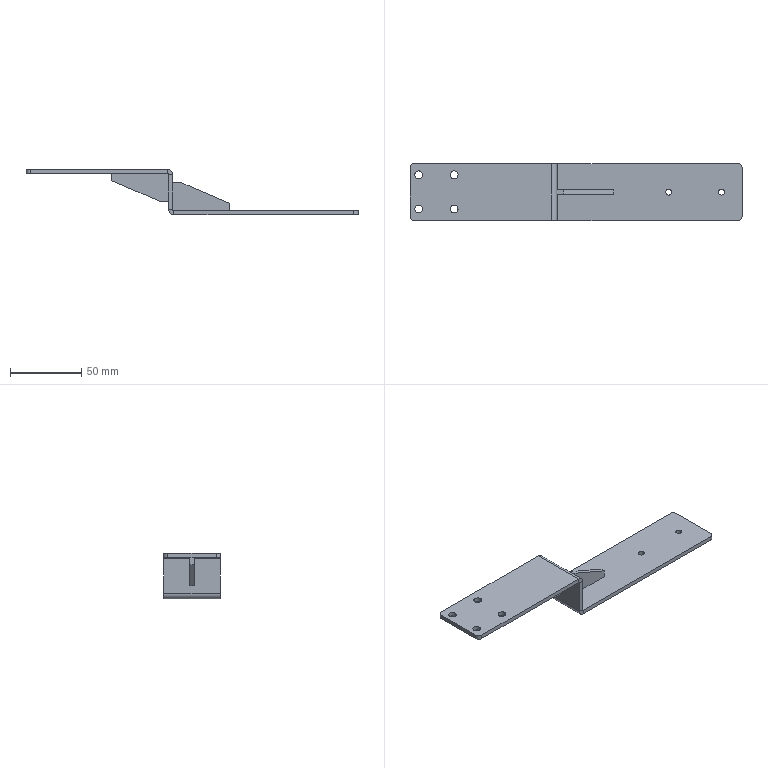Part | SolidWorks | features HoleWzd 2, ICE 2, Fillet 1, FlatPattern 1, SMBaseFlange 1, SheetMetal 1 | 1 solid | 50 faces | box 233 x 40 x 32 mm | volume 34041 mm3 | plane 28 | cylinder 22 | commonest cylinder face diameters 5.5 x8 1.5 x4 4.2 x4 6 x4 7.5 x2
STEP:
#1=CARTESIAN_POINT('',(8.75,8.,0.));
#2=VERTEX_POINT('',#1);
#3=CARTESIAN_POINT('',(3.25,8.,0.));
#4=VERTEX_POINT('',#3);
#5=CARTESIAN_POINT('',(6.,8.,0.));
#6=DIRECTION('',(0.,0.,-1.));
#7=DIRECTION('',(-1.,0.,0.));
#8=AXIS2_PLACEMENT_3D('',#5,#6,#7);
#9=CIRCLE('',#8,2.75);
#10=EDGE_CURVE('',#2,#4,#9,.T.);
#11=ORIENTED_EDGE('',*,*,#10,.T.);
#12=CARTESIAN_POINT('',(3.25,8.,3.));
#13=VERTEX_POINT('',#12);
#14=CARTESIAN_POINT('',(3.25,8.,3.));
#15=DIRECTION('',(0.,0.,1.));
#16=VECTOR('',#15,1000.);
#17=LINE('',#14,#16);
#18=EDGE_CURVE('',#4,#13,#17,.T.);
#19=ORIENTED_EDGE('',*,*,#18,.T.);
#20=CARTESIAN_POINT('',(8.75,8.,3.));
#21=VERTEX_POINT('',#20);
#22=CARTESIAN_POINT('',(6.,8.,3.));
#23=DIRECTION('',(0.,0.,1.));
#24=DIRECTION('',(1.,0.,0.));
#25=AXIS2_PLACEMENT_3D('',#22,#23,#24);
#26=CIRCLE('',#25,2.75);
#27=EDGE_CURVE('',#13,#21,#26,.T.);
#28=ORIENTED_EDGE('',*,*,#27,.T.);
#29=CARTESIAN_POINT('',(8.75,8.,3.));
#30=DIRECTION('',(0.,0.,1.));
#31=VECTOR('',#30,1000.);
#32=LINE('',#29,#31);
#33=EDGE_CURVE('',#2,#21,#32,.T.);
#34=ORIENTED_EDGE('',*,*,#33,.F.);
#35=EDGE_LOOP('',(#11,#19,#28,#34));
#36=FACE_OUTER_BOUND('',#35,.T.);
#37=CARTESIAN_POINT('',(6.,8.,3.));
#38=DIRECTION('',(0.,0.,1.));
#39=DIRECTION('',(1.,0.,0.));
#40=AXIS2_PLACEMENT_3D('',#37,#38,#39);
#41=CYLINDRICAL_SURFACE('',#40,2.75);
#42=ADVANCED_FACE('',(#36),#41,.F.);
#43=CARTESIAN_POINT('',(8.75,32.,0.));
#44=VERTEX_POINT('',#43);
#45=CARTESIAN_POINT('',(3.25,32.,0.));
#46=VERTEX_POINT('',#45);
#47=CARTESIAN_POINT('',(6.,32.,0.));
#48=DIRECTION('',(0.,0.,-1.));
#49=DIRECTION('',(-1.,0.,0.));
#50=AXIS2_PLACEMENT_3D('',#47,#48,#49);
#51=CIRCLE('',#50,2.75);
#52=EDGE_CURVE('',#44,#46,#51,.T.);
#53=ORIENTED_EDGE('',*,*,#52,.T.);
#54=CARTESIAN_POINT('',(3.25,32.,3.));
#55=VERTEX_POINT('',#54);
#56=CARTESIAN_POINT('',(3.25,32.,3.));
#57=DIRECTION('',(0.,0.,1.));
#58=VECTOR('',#57,1000.);
#59=LINE('',#56,#58);
#60=EDGE_CURVE('',#46,#55,#59,.T.);
#61=ORIENTED_EDGE('',*,*,#60,.T.);
#62=CARTESIAN_POINT('',(8.75,32.,3.));
#63=VERTEX_POINT('',#62);
#64=CARTESIAN_POINT('',(6.,32.,3.));
#65=DIRECTION('',(0.,0.,1.));
#66=DIRECTION('',(1.,0.,0.));
#67=AXIS2_PLACEMENT_3D('',#64,#65,#66);
#68=CIRCLE('',#67,2.75);
#69=EDGE_CURVE('',#55,#63,#68,.T.);
#70=ORIENTED_EDGE('',*,*,#69,.T.);
#71=CARTESIAN_POINT('',(8.75,32.,3.));
#72=DIRECTION('',(0.,0.,1.));
#73=VECTOR('',#72,1000.);
#74=LINE('',#71,#73);
#75=EDGE_CURVE('',#44,#63,#74,.T.);
#76=ORIENTED_EDGE('',*,*,#75,.F.);
#77=EDGE_LOOP('',(#53,#61,#70,#76));
#78=FACE_OUTER_BOUND('',#77,.T.);
#79=CARTESIAN_POINT('',(6.,32.,3.));
#80=DIRECTION('',(0.,0.,1.));
#81=DIRECTION('',(1.,0.,0.));
#82=AXIS2_PLACEMENT_3D('',#79,#80,#81);
#83=CYLINDRICAL_SURFACE('',#82,2.75);
#84=ADVANCED_FACE('',(#78),#83,.F.);
#85=CARTESIAN_POINT('',(33.75,8.,0.));
#86=VERTEX_POINT('',#85);
#87=CARTESIAN_POINT('',(28.25,8.,0.));
#88=VERTEX_POINT('',#87);
#89=CARTESIAN_POINT('',(31.,8.,0.));
#90=DIRECTION('',(0.,0.,-1.));
#91=DIRECTION('',(-1.,0.,0.));
#92=AXIS2_PLACEMENT_3D('',#89,#90,#91);
#93=CIRCLE('',#92,2.75);
#94=EDGE_CURVE('',#86,#88,#93,.T.);
#95=ORIENTED_EDGE('',*,*,#94,.T.);
#96=CARTESIAN_POINT('',(28.25,8.,3.));
#97=VERTEX_POINT('',#96);
#98=CARTESIAN_POINT('',(28.25,8.,3.));
#99=DIRECTION('',(0.,0.,1.));
#100=VECTOR('',#99,1000.);
#101=LINE('',#98,#100);
#102=EDGE_CURVE('',#88,#97,#101,.T.);
#103=ORIENTED_EDGE('',*,*,#102,.T.);
#104=CARTESIAN_POINT('',(33.75,8.,3.));
#105=VERTEX_POINT('',#104);
#106=CARTESIAN_POINT('',(31.,8.,3.));
#107=DIRECTION('',(0.,0.,1.));
#108=DIRECTION('',(1.,0.,0.));
#109=AXIS2_PLACEMENT_3D('',#106,#107,#108);
#110=CIRCLE('',#109,2.75);
#111=EDGE_CURVE('',#97,#105,#110,.T.);
#112=ORIENTED_EDGE('',*,*,#111,.T.);
#113=CARTESIAN_POINT('',(33.75,8.,3.));
#114=DIRECTION('',(0.,0.,1.));
#115=VECTOR('',#114,1000.);
#116=LINE('',#113,#115);
#117=EDGE_CURVE('',#86,#105,#116,.T.);
#118=ORIENTED_EDGE('',*,*,#117,.F.);
#119=EDGE_LOOP('',(#95,#103,#112,#118));
#120=FACE_OUTER_BOUND('',#119,.T.);
#121=CARTESIAN_POINT('',(31.,8.,3.));
#122=DIRECTION('',(0.,0.,1.));
#123=DIRECTION('',(1.,0.,0.));
#124=AXIS2_PLACEMENT_3D('',#121,#122,#123);
#125=CYLINDRICAL_SURFACE('',#124,2.75);
#126=ADVANCED_FACE('',(#120),#125,.F.);
#127=CARTESIAN_POINT('',(33.75,32.,0.));
#128=VERTEX_POINT('',#127);
#129=CARTESIAN_POINT('',(28.25,32.,0.));
#130=VERTEX_POINT('',#129);
#131=CARTESIAN_POINT('',(31.,32.,0.));
#132=DIRECTION('',(0.,0.,-1.));
#133=DIRECTION('',(-1.,0.,0.));
#134=AXIS2_PLACEMENT_3D('',#131,#132,#133);
#135=CIRCLE('',#134,2.75);
#136=EDGE_CURVE('',#128,#130,#135,.T.);
#137=ORIENTED_EDGE('',*,*,#136,.T.);
#138=CARTESIAN_POINT('',(28.25,32.,3.));
#139=VERTEX_POINT('',#138);
#140=CARTESIAN_POINT('',(28.25,32.,3.));
#141=DIRECTION('',(0.,0.,1.));
#142=VECTOR('',#141,1000.);
#143=LINE('',#140,#142);
#144=EDGE_CURVE('',#130,#139,#143,.T.);
#145=ORIENTED_EDGE('',*,*,#144,.T.);
#146=CARTESIAN_POINT('',(33.75,32.,3.));
#147=VERTEX_POINT('',#146);
#148=CARTESIAN_POINT('',(31.,32.,3.));
#149=DIRECTION('',(0.,0.,1.));
#150=DIRECTION('',(1.,0.,0.));
#151=AXIS2_PLACEMENT_3D('',#148,#149,#150);
#152=CIRCLE('',#151,2.75);
#153=EDGE_CURVE('',#139,#147,#152,.T.);
#154=ORIENTED_EDGE('',*,*,#153,.T.);
#155=CARTESIAN_POINT('',(33.75,32.,3.));
#156=DIRECTION('',(0.,0.,1.));
#157=VECTOR('',#156,1000.);
#158=LINE('',#155,#157);
#159=EDGE_CURVE('',#128,#147,#158,.T.);
#160=ORIENTED_EDGE('',*,*,#159,.F.);
#161=EDGE_LOOP('',(#137,#145,#154,#160));
#162=FACE_OUTER_BOUND('',#161,.T.);
#163=CARTESIAN_POINT('',(31.,32.,3.));
#164=DIRECTION('',(0.,0.,1.));
#165=DIRECTION('',(1.,0.,0.));
#166=AXIS2_PLACEMENT_3D('',#163,#164,#165);
#167=CYLINDRICAL_SURFACE('',#166,2.75);
#168=ADVANCED_FACE('',(#162),#167,.F.);
#169=CARTESIAN_POINT('',(220.65,20.,-29.));
#170=VERTEX_POINT('',#169);
#171=CARTESIAN_POINT('',(216.45,20.,-29.));
#172=VERTEX_POINT('',#171);
#173=CARTESIAN_POINT('',(218.55,20.,-29.));
#174=DIRECTION('',(0.,0.,-1.));
#175=DIRECTION('',(-1.,0.,0.));
#176=AXIS2_PLACEMENT_3D('',#173,#174,#175);
#177=CIRCLE('',#176,2.1);
#178=EDGE_CURVE('',#170,#172,#177,.T.);
#179=ORIENTED_EDGE('',*,*,#178,.T.);
#180=CARTESIAN_POINT('',(216.45,20.,-26.));
#181=VERTEX_POINT('',#180);
#182=CARTESIAN_POINT('',(216.45,20.,-26.));
#183=DIRECTION('',(0.,0.,1.));
#184=VECTOR('',#183,1000.);
#185=LINE('',#182,#184);
#186=EDGE_CURVE('',#172,#181,#185,.T.);
#187=ORIENTED_EDGE('',*,*,#186,.T.);
#188=CARTESIAN_POINT('',(220.65,20.,-26.));
#189=VERTEX_POINT('',#188);
#190=CARTESIAN_POINT('',(218.55,20.,-26.));
#191=DIRECTION('',(0.,0.,1.));
#192=DIRECTION('',(1.,0.,0.));
#193=AXIS2_PLACEMENT_3D('',#190,#191,#192);
#194=CIRCLE('',#193,2.1);
#195=EDGE_CURVE('',#181,#189,#194,.T.);
#196=ORIENTED_EDGE('',*,*,#195,.T.);
#197=CARTESIAN_POINT('',(220.65,20.,-26.));
#198=DIRECTION('',(0.,0.,1.));
#199=VECTOR('',#198,1000.);
#200=LINE('',#197,#199);
#201=EDGE_CURVE('',#170,#189,#200,.T.);
#202=ORIENTED_EDGE('',*,*,#201,.F.);
#203=EDGE_LOOP('',(#179,#187,#196,#202));
#204=FACE_OUTER_BOUND('',#203,.T.);
#205=CARTESIAN_POINT('',(218.55,20.,-26.));
#206=DIRECTION('',(0.,0.,1.));
#207=DIRECTION('',(1.,0.,0.));
#208=AXIS2_PLACEMENT_3D('',#205,#206,#207);
#209=CYLINDRICAL_SURFACE('',#208,2.1);
#210=ADVANCED_FACE('',(#204),#209,.F.);
#211=CARTESIAN_POINT('',(183.65,20.,-29.));
#212=VERTEX_POINT('',#211);
#213=CARTESIAN_POINT('',(179.45,20.,-29.));
#214=VERTEX_POINT('',#213);
#215=CARTESIAN_POINT('',(181.55,20.,-29.));
#216=DIRECTION('',(0.,0.,-1.));
#217=DIRECTION('',(-1.,0.,0.));
#218=AXIS2_PLACEMENT_3D('',#215,#216,#217);
#219=CIRCLE('',#218,2.1);
#220=EDGE_CURVE('',#212,#214,#219,.T.);
#221=ORIENTED_EDGE('',*,*,#220,.T.);
#222=CARTESIAN_POINT('',(179.45,20.,-26.));
#223=VERTEX_POINT('',#222);
#224=CARTESIAN_POINT('',(179.45,20.,-26.));
#225=DIRECTION('',(0.,0.,1.));
#226=VECTOR('',#225,1000.);
#227=LINE('',#224,#226);
#228=EDGE_CURVE('',#214,#223,#227,.T.);
#229=ORIENTED_EDGE('',*,*,#228,.T.);
#230=CARTESIAN_POINT('',(183.65,20.,-26.));
#231=VERTEX_POINT('',#230);
#232=CARTESIAN_POINT('',(181.55,20.,-26.));
#233=DIRECTION('',(0.,0.,1.));
#234=DIRECTION('',(1.,0.,0.));
#235=AXIS2_PLACEMENT_3D('',#232,#233,#234);
#236=CIRCLE('',#235,2.1);
#237=EDGE_CURVE('',#223,#231,#236,.T.);
#238=ORIENTED_EDGE('',*,*,#237,.T.);
#239=CARTESIAN_POINT('',(183.65,20.,-26.));
#240=DIRECTION('',(0.,0.,1.));
#241=VECTOR('',#240,1000.);
#242=LINE('',#239,#241);
#243=EDGE_CURVE('',#212,#231,#242,.T.);
#244=ORIENTED_EDGE('',*,*,#243,.F.);
#245=EDGE_LOOP('',(#221,#229,#238,#244));
#246=FACE_OUTER_BOUND('',#245,.T.);
#247=CARTESIAN_POINT('',(181.55,20.,-26.));
#248=DIRECTION('',(0.,0.,1.));
#249=DIRECTION('',(1.,0.,0.));
#250=AXIS2_PLACEMENT_3D('',#247,#248,#249);
#251=CYLINDRICAL_SURFACE('',#250,2.1);
#252=ADVANCED_FACE('',(#246),#251,.F.);
#253=CARTESIAN_POINT('',(103.75,18.5,-26.));
#254=VERTEX_POINT('',#253);
#255=CARTESIAN_POINT('',(103.,18.5,-25.25));
#256=VERTEX_POINT('',#255);
#257=CARTESIAN_POINT('',(103.75,18.5,-25.25));
#258=DIRECTION('',(0.,1.,0.));
#259=DIRECTION('',(0.,0.,1.));
#260=AXIS2_PLACEMENT_3D('',#257,#258,#259);
#261=CIRCLE('',#260,0.75);
#262=EDGE_CURVE('',#254,#256,#261,.T.);
#263=ORIENTED_EDGE('',*,*,#262,.T.);
#264=CARTESIAN_POINT('',(103.,0.,-25.25));
#265=VERTEX_POINT('',#264);
#266=CARTESIAN_POINT('',(103.,40.,-25.25));
#267=DIRECTION('',(0.,-1.,0.));
#268=VECTOR('',#267,1000.);
#269=LINE('',#266,#268);
#270=EDGE_CURVE('',#256,#265,#269,.T.);
#271=ORIENTED_EDGE('',*,*,#270,.T.);
#272=CARTESIAN_POINT('',(103.75,0.,-26.));
#273=VERTEX_POINT('',#272);
#274=CARTESIAN_POINT('',(103.75,0.,-25.25));
#275=DIRECTION('',(0.,-1.,0.));
#276=DIRECTION('',(1.,0.,0.));
#277=AXIS2_PLACEMENT_3D('',#274,#275,#276);
#278=CIRCLE('',#277,0.75);
#279=EDGE_CURVE('',#265,#273,#278,.T.);
#280=ORIENTED_EDGE('',*,*,#279,.T.);
#281=CARTESIAN_POINT('',(103.75,40.,-26.));
#282=DIRECTION('',(0.,-1.,0.));
#283=VECTOR('',#282,1000.);
#284=LINE('',#281,#283);
#285=EDGE_CURVE('',#254,#273,#284,.T.);
#286=ORIENTED_EDGE('',*,*,#285,.F.);
#287=EDGE_LOOP('',(#263,#271,#280,#286));
#288=FACE_OUTER_BOUND('',#287,.T.);
#289=CARTESIAN_POINT('',(103.75,40.,-25.25));
#290=DIRECTION('',(0.,-1.,0.));
#291=DIRECTION('',(0.,0.,-1.));
#292=AXIS2_PLACEMENT_3D('',#289,#290,#291);
#293=CYLINDRICAL_SURFACE('',#292,0.75);
#294=ADVANCED_FACE('',(#288),#293,.F.);
#295=CARTESIAN_POINT('',(99.25,18.5,0.));
#296=VERTEX_POINT('',#295);
#297=CARTESIAN_POINT('',(99.25,0.,0.));
#298=VERTEX_POINT('',#297);
#299=CARTESIAN_POINT('',(99.25,40.,0.));
#300=DIRECTION('',(0.,-1.,0.));
#301=VECTOR('',#300,1000.);
#302=LINE('',#299,#301);
#303=EDGE_CURVE('',#296,#298,#302,.T.);
#304=ORIENTED_EDGE('',*,*,#303,.F.);
#305=CARTESIAN_POINT('',(100.,18.5,-0.75));
#306=VERTEX_POINT('',#305);
#307=CARTESIAN_POINT('',(99.25,18.5,-0.75));
#308=DIRECTION('',(0.,1.,0.));
#309=DIRECTION('',(0.,0.,1.));
#310=AXIS2_PLACEMENT_3D('',#307,#308,#309);
#311=CIRCLE('',#310,0.75);
#312=EDGE_CURVE('',#296,#306,#311,.T.);
#313=ORIENTED_EDGE('',*,*,#312,.T.);
#314=CARTESIAN_POINT('',(100.,0.,-0.75));
#315=VERTEX_POINT('',#314);
#316=CARTESIAN_POINT('',(100.,40.,-0.75));
#317=DIRECTION('',(0.,-1.,0.));
#318=VECTOR('',#317,1000.);
#319=LINE('',#316,#318);
#320=EDGE_CURVE('',#306,#315,#319,.T.);
#321=ORIENTED_EDGE('',*,*,#320,.T.);
#322=CARTESIAN_POINT('',(99.25,0.,-0.75));
#323=DIRECTION('',(0.,1.,0.));
#324=DIRECTION('',(0.,0.,-1.));
#325=AXIS2_PLACEMENT_3D('',#322,#323,#324);
#326=CIRCLE('',#325,0.75);
#327=EDGE_CURVE('',#298,#315,#326,.T.);
#328=ORIENTED_EDGE('',*,*,#327,.F.);
#329=EDGE_LOOP('',(#304,#313,#321,#328));
#330=FACE_OUTER_BOUND('',#329,.T.);
#331=CARTESIAN_POINT('',(99.25,40.,-0.75));
#332=DIRECTION('',(0.,-1.,0.));
#333=DIRECTION('',(0.,0.,-1.));
#334=AXIS2_PLACEMENT_3D('',#331,#332,#333);
#335=CYLINDRICAL_SURFACE('',#334,0.75);
#336=ADVANCED_FACE('',(#330),#335,.F.);
#337=CARTESIAN_POINT('',(100.,40.,-0.75));
#338=VERTEX_POINT('',#337);
#339=CARTESIAN_POINT('',(103.,40.,-0.75));
#340=VERTEX_POINT('',#339);
#341=CARTESIAN_POINT('',(100.,40.,-0.75));
#342=DIRECTION('',(1.,0.,0.));
#343=VECTOR('',#342,1000.);
#344=LINE('',#341,#343);
#345=EDGE_CURVE('',#338,#340,#344,.T.);
#346=ORIENTED_EDGE('',*,*,#345,.F.);
#347=CARTESIAN_POINT('',(99.25,40.,0.));
#348=VERTEX_POINT('',#347);
#349=CARTESIAN_POINT('',(99.25,40.,-0.75));
#350=DIRECTION('',(0.,1.,0.));
#351=DIRECTION('',(0.,0.,-1.));
#352=AXIS2_PLACEMENT_3D('',#349,#350,#351);
#353=CIRCLE('',#352,0.75);
#354=EDGE_CURVE('',#348,#338,#353,.T.);
#355=ORIENTED_EDGE('',*,*,#354,.F.);
#356=CARTESIAN_POINT('',(99.25,40.,3.));
#357=VERTEX_POINT('',#356);
#358=CARTESIAN_POINT('',(99.25,40.,3.));
#359=DIRECTION('',(0.,0.,-1.));
#360=VECTOR('',#359,1000.);
#361=LINE('',#358,#360);
#362=EDGE_CURVE('',#357,#348,#361,.T.);
#363=ORIENTED_EDGE('',*,*,#362,.F.);
#364=CARTESIAN_POINT('',(99.25,40.,-0.75));
#365=DIRECTION('',(0.,1.,0.));
#366=DIRECTION('',(1.,0.,0.));
#367=AXIS2_PLACEMENT_3D('',#364,#365,#366);
#368=CIRCLE('',#367,3.75);
#369=EDGE_CURVE('',#357,#340,#368,.T.);
#370=ORIENTED_EDGE('',*,*,#369,.T.);
#371=EDGE_LOOP('',(#346,#355,#363,#370));
#372=FACE_OUTER_BOUND('',#371,.T.);
#373=CARTESIAN_POINT('',(100.,40.,-0.75));
#374=DIRECTION('',(0.,1.,0.));
#375=DIRECTION('',(0.,0.,1.));
#376=AXIS2_PLACEMENT_3D('',#373,#374,#375);
#377=PLANE('',#376);
#378=ADVANCED_FACE('',(#372),#377,.T.);
#379=CARTESIAN_POINT('',(100.,40.,-25.25));
#380=VERTEX_POINT('',#379);
#381=CARTESIAN_POINT('',(100.,40.,0.));
#382=DIRECTION('',(0.,0.,-1.));
#383=VECTOR('',#382,1000.);
#384=LINE('',#381,#383);
#385=EDGE_CURVE('',#338,#380,#384,.T.);
#386=ORIENTED_EDGE('',*,*,#385,.F.);
#387=ORIENTED_EDGE('',*,*,#345,.T.);
#388=CARTESIAN_POINT('',(103.,40.,-25.25));
#389=VERTEX_POINT('',#388);
#390=CARTESIAN_POINT('',(103.,40.,0.));
#391=DIRECTION('',(0.,0.,-1.));
#392=VECTOR('',#391,1000.);
#393=LINE('',#390,#392);
#394=EDGE_CURVE('',#340,#389,#393,.T.);
#395=ORIENTED_EDGE('',*,*,#394,.T.);
#396=CARTESIAN_POINT('',(103.,40.,-25.25));
#397=DIRECTION('',(-1.,0.,0.));
#398=VECTOR('',#397,1000.);
#399=LINE('',#396,#398);
#400=EDGE_CURVE('',#389,#380,#399,.T.);
#401=ORIENTED_EDGE('',*,*,#400,.T.);
#402=EDGE_LOOP('',(#386,#387,#395,#401));
#403=FACE_OUTER_BOUND('',#402,.T.);
#404=CARTESIAN_POINT('',(99.25,40.,3.));
#405=DIRECTION('',(0.,1.,0.));
#406=DIRECTION('',(0.,0.,1.));
#407=AXIS2_PLACEMENT_3D('',#404,#405,#406);
#408=PLANE('',#407);
#409=ADVANCED_FACE('',(#403),#408,.T.);
#410=CARTESIAN_POINT('',(99.25,0.,3.));
#411=VERTEX_POINT('',#410);
#412=CARTESIAN_POINT('',(99.25,0.,0.));
#413=DIRECTION('',(0.,0.,1.));
#414=VECTOR('',#413,1000.);
#415=LINE('',#412,#414);
#416=EDGE_CURVE('',#298,#411,#415,.T.);
#417=ORIENTED_EDGE('',*,*,#416,.F.);
#418=ORIENTED_EDGE('',*,*,#327,.T.);
#419=CARTESIAN_POINT('',(103.,0.,-0.75));
#420=VERTEX_POINT('',#419);
#421=CARTESIAN_POINT('',(103.,0.,-0.75));
#422=DIRECTION('',(-1.,0.,0.));
#423=VECTOR('',#422,1000.);
#424=LINE('',#421,#423);
#425=EDGE_CURVE('',#420,#315,#424,.T.);
#426=ORIENTED_EDGE('',*,*,#425,.F.);
#427=CARTESIAN_POINT('',(99.25,0.,-0.75));
#428=DIRECTION('',(0.,1.,0.));
#429=DIRECTION('',(1.,0.,0.));
#430=AXIS2_PLACEMENT_3D('',#427,#428,#429);
#431=CIRCLE('',#430,3.75);
#432=EDGE_CURVE('',#411,#420,#431,.T.);
#433=ORIENTED_EDGE('',*,*,#432,.F.);
#434=EDGE_LOOP('',(#417,#418,#426,#433));
#435=FACE_OUTER_BOUND('',#434,.T.);
#436=CARTESIAN_POINT('',(99.25,0.,0.));
#437=DIRECTION('',(0.,-1.,0.));
#438=DIRECTION('',(0.,0.,-1.));
#439=AXIS2_PLACEMENT_3D('',#436,#437,#438);
#440=PLANE('',#439);
#441=ADVANCED_FACE('',(#435),#440,.T.);
#442=CARTESIAN_POINT('',(3.,0.,3.));
#443=VERTEX_POINT('',#442);
#444=CARTESIAN_POINT('',(0.,0.,3.));
#445=DIRECTION('',(1.,0.,0.));
#446=VECTOR('',#445,1000.);
#447=LINE('',#444,#446);
#448=EDGE_CURVE('',#443,#411,#447,.T.);
#449=ORIENTED_EDGE('',*,*,#448,.F.);
#450=CARTESIAN_POINT('',(3.,0.,0.));
#451=VERTEX_POINT('',#450);
#452=CARTESIAN_POINT('',(3.,0.,-0.75));
#453=DIRECTION('',(0.,0.,-1.));
#454=VECTOR('',#453,1000.);
#455=LINE('',#452,#454);
#456=EDGE_CURVE('',#443,#451,#455,.T.);
#457=ORIENTED_EDGE('',*,*,#456,.T.);
#458=CARTESIAN_POINT('',(0.,0.,0.));
#459=DIRECTION('',(1.,0.,0.));
#460=VECTOR('',#459,1000.);
#461=LINE('',#458,#460);
#462=EDGE_CURVE('',#451,#298,#461,.T.);
#463=ORIENTED_EDGE('',*,*,#462,.T.);
#464=ORIENTED_EDGE('',*,*,#416,.T.);
#465=EDGE_LOOP('',(#449,#457,#463,#464));
#466=FACE_OUTER_BOUND('',#465,.T.);
#467=CARTESIAN_POINT('',(103.,0.,-0.75));
#468=DIRECTION('',(0.,-1.,0.));
#469=DIRECTION('',(0.,0.,-1.));
#470=AXIS2_PLACEMENT_3D('',#467,#468,#469);
#471=PLANE('',#470);
#472=ADVANCED_FACE('',(#466),#471,.T.);
#473=CARTESIAN_POINT('',(103.75,40.,-29.));
#474=VERTEX_POINT('',#473);
#475=CARTESIAN_POINT('',(103.75,40.,-26.));
#476=VERTEX_POINT('',#475);
#477=CARTESIAN_POINT('',(103.75,40.,-29.));
#478=DIRECTION('',(0.,0.,1.));
#479=VECTOR('',#478,1000.);
#480=LINE('',#477,#479);
#481=EDGE_CURVE('',#474,#476,#480,.T.);
#482=ORIENTED_EDGE('',*,*,#481,.F.);
#483=CARTESIAN_POINT('',(103.75,40.,-25.25));
#484=DIRECTION('',(0.,-1.,0.));
#485=DIRECTION('',(0.,0.,1.));
#486=AXIS2_PLACEMENT_3D('',#483,#484,#485);
#487=CIRCLE('',#486,3.75);
#488=EDGE_CURVE('',#380,#474,#487,.T.);
#489=ORIENTED_EDGE('',*,*,#488,.F.);
#490=ORIENTED_EDGE('',*,*,#400,.F.);
#491=CARTESIAN_POINT('',(103.75,40.,-25.25));
#492=DIRECTION('',(0.,-1.,0.));
#493=DIRECTION('',(1.,0.,0.));
#494=AXIS2_PLACEMENT_3D('',#491,#492,#493);
#495=CIRCLE('',#494,0.75);
#496=EDGE_CURVE('',#389,#476,#495,.T.);
#497=ORIENTED_EDGE('',*,*,#496,.T.);
#498=EDGE_LOOP('',(#482,#489,#490,#497));
#499=FACE_OUTER_BOUND('',#498,.T.);
#500=CARTESIAN_POINT('',(103.75,40.,-29.));
#501=DIRECTION('',(0.,1.,0.));
#502=DIRECTION('',(0.,0.,1.));
#503=AXIS2_PLACEMENT_3D('',#500,#501,#502);
#504=PLANE('',#503);
#505=ADVANCED_FACE('',(#499),#504,.T.);
#506=CARTESIAN_POINT('',(230.,40.,-26.));
#507=VERTEX_POINT('',#506);
#508=CARTESIAN_POINT('',(100.,40.,-26.));
#509=DIRECTION('',(1.,0.,0.));
#510=VECTOR('',#509,1000.);
#511=LINE('',#508,#510);
#512=EDGE_CURVE('',#476,#507,#511,.T.);
#513=ORIENTED_EDGE('',*,*,#512,.T.);
#514=CARTESIAN_POINT('',(230.,40.,-29.));
#515=VERTEX_POINT('',#514);
#516=CARTESIAN_POINT('',(230.,40.,-25.25));
#517=DIRECTION('',(0.,0.,-1.));
#518=VECTOR('',#517,1000.);
#519=LINE('',#516,#518);
#520=EDGE_CURVE('',#507,#515,#519,.T.);
#521=ORIENTED_EDGE('',*,*,#520,.T.);
#522=CARTESIAN_POINT('',(100.,40.,-29.));
#523=DIRECTION('',(1.,0.,0.));
#524=VECTOR('',#523,1000.);
#525=LINE('',#522,#524);
#526=EDGE_CURVE('',#474,#515,#525,.T.);
#527=ORIENTED_EDGE('',*,*,#526,.F.);
#528=ORIENTED_EDGE('',*,*,#481,.T.);
#529=EDGE_LOOP('',(#513,#521,#527,#528));
#530=FACE_OUTER_BOUND('',#529,.T.);
#531=CARTESIAN_POINT('',(103.,40.,-25.25));
#532=DIRECTION('',(0.,1.,0.));
#533=DIRECTION('',(0.,0.,1.));
#534=AXIS2_PLACEMENT_3D('',#531,#532,#533);
#535=PLANE('',#534);
#536=ADVANCED_FACE('',(#530),#535,.T.);
#537=CARTESIAN_POINT('',(100.,0.,-25.25));
#538=VERTEX_POINT('',#537);
#539=CARTESIAN_POINT('',(100.,0.,-25.25));
#540=DIRECTION('',(1.,0.,0.));
#541=VECTOR('',#540,1000.);
#542=LINE('',#539,#541);
#543=EDGE_CURVE('',#538,#265,#542,.T.);
#544=ORIENTED_EDGE('',*,*,#543,.F.);
#545=CARTESIAN_POINT('',(103.75,0.,-29.));
#546=VERTEX_POINT('',#545);
#547=CARTESIAN_POINT('',(103.75,0.,-25.25));
#548=DIRECTION('',(0.,-1.,0.));
#549=DIRECTION('',(0.,0.,1.));
#550=AXIS2_PLACEMENT_3D('',#547,#548,#549);
#551=CIRCLE('',#550,3.75);
#552=EDGE_CURVE('',#538,#546,#551,.T.);
#553=ORIENTED_EDGE('',*,*,#552,.T.);
#554=CARTESIAN_POINT('',(103.75,0.,-26.));
#555=DIRECTION('',(0.,0.,-1.));
#556=VECTOR('',#555,1000.);
#557=LINE('',#554,#556);
#558=EDGE_CURVE('',#273,#546,#557,.T.);
#559=ORIENTED_EDGE('',*,*,#558,.F.);
#560=ORIENTED_EDGE('',*,*,#279,.F.);
#561=EDGE_LOOP('',(#544,#553,#559,#560));
#562=FACE_OUTER_BOUND('',#561,.T.);
#563=CARTESIAN_POINT('',(100.,0.,-25.25));
#564=DIRECTION('',(0.,-1.,0.));
#565=DIRECTION('',(0.,0.,-1.));
#566=AXIS2_PLACEMENT_3D('',#563,#564,#565);
#567=PLANE('',#566);
#568=ADVANCED_FACE('',(#562),#567,.T.);
#569=CARTESIAN_POINT('',(100.,0.,0.));
#570=DIRECTION('',(0.,0.,-1.));
#571=VECTOR('',#570,1000.);
#572=LINE('',#569,#571);
#573=EDGE_CURVE('',#315,#538,#572,.T.);
#574=ORIENTED_EDGE('',*,*,#573,.T.);
#575=ORIENTED_EDGE('',*,*,#543,.T.);
#576=CARTESIAN_POINT('',(103.,0.,0.));
#577=DIRECTION('',(0.,0.,-1.));
#578=VECTOR('',#577,1000.);
#579=LINE('',#576,#578);
#580=EDGE_CURVE('',#420,#265,#579,.T.);
#581=ORIENTED_EDGE('',*,*,#580,.F.);
#582=ORIENTED_EDGE('',*,*,#425,.T.);
#583=EDGE_LOOP('',(#574,#575,#581,#582));
#584=FACE_OUTER_BOUND('',#583,.T.);
#585=CARTESIAN_POINT('',(103.75,0.,-26.));
#586=DIRECTION('',(0.,-1.,0.));
#587=DIRECTION('',(0.,0.,-1.));
#588=AXIS2_PLACEMENT_3D('',#585,#586,#587);
#589=PLANE('',#588);
#590=ADVANCED_FACE('',(#584),#589,.T.);
#591=CARTESIAN_POINT('',(218.55,20.,-26.));
#592=DIRECTION('',(0.,0.,1.));
#593=DIRECTION('',(1.,0.,0.));
#594=AXIS2_PLACEMENT_3D('',#591,#592,#593);
#595=CIRCLE('',#594,2.1);
#596=EDGE_CURVE('',#189,#181,#595,.T.);
#597=ORIENTED_EDGE('',*,*,#596,.F.);
#598=ORIENTED_EDGE('',*,*,#195,.F.);
#599=EDGE_LOOP('',(#597,#598));
#600=FACE_BOUND('',#599,.T.);
#601=CARTESIAN_POINT('',(181.55,20.,-26.));
#602=DIRECTION('',(0.,0.,1.));
#603=DIRECTION('',(1.,0.,0.));
#604=AXIS2_PLACEMENT_3D('',#601,#602,#603);
#605=CIRCLE('',#604,2.1);
#606=EDGE_CURVE('',#231,#223,#605,.T.);
#607=ORIENTED_EDGE('',*,*,#606,.F.);
#608=ORIENTED_EDGE('',*,*,#237,.F.);
#609=EDGE_LOOP('',(#607,#608));
#610=FACE_BOUND('',#609,.T.);
#611=CARTESIAN_POINT('',(103.75,21.5,-26.));
#612=VERTEX_POINT('',#611);
#613=CARTESIAN_POINT('',(103.75,40.,-26.));
#614=DIRECTION('',(0.,-1.,0.));
#615=VECTOR('',#614,1000.);
#616=LINE('',#613,#615);
#617=EDGE_CURVE('',#476,#612,#616,.T.);
#618=ORIENTED_EDGE('',*,*,#617,.T.);
#619=CARTESIAN_POINT('',(143.,21.5,-26.));
#620=VERTEX_POINT('',#619);
#621=CARTESIAN_POINT('',(103.75,21.5,-26.));
#622=DIRECTION('',(-1.,0.,0.));
#623=VECTOR('',#622,1000.);
#624=LINE('',#621,#623);
#625=EDGE_CURVE('',#620,#612,#624,.T.);
#626=ORIENTED_EDGE('',*,*,#625,.F.);
#627=CARTESIAN_POINT('',(143.,18.5,-26.));
#628=VERTEX_POINT('',#627);
#629=CARTESIAN_POINT('',(143.,21.5,-26.));
#630=DIRECTION('',(0.,-1.,0.));
#631=VECTOR('',#630,1000.);
#632=LINE('',#629,#631);
#633=EDGE_CURVE('',#620,#628,#632,.T.);
#634=ORIENTED_EDGE('',*,*,#633,.T.);
#635=CARTESIAN_POINT('',(103.75,18.5,-26.));
#636=DIRECTION('',(-1.,0.,0.));
#637=VECTOR('',#636,1000.);
#638=LINE('',#635,#637);
#639=EDGE_CURVE('',#628,#254,#638,.T.);
#640=ORIENTED_EDGE('',*,*,#639,.T.);
#641=ORIENTED_EDGE('',*,*,#285,.T.);
#642=CARTESIAN_POINT('',(230.,0.,-26.));
#643=VERTEX_POINT('',#642);
#644=CARTESIAN_POINT('',(100.,0.,-26.));
#645=DIRECTION('',(1.,0.,0.));
#646=VECTOR('',#645,1000.);
#647=LINE('',#644,#646);
#648=EDGE_CURVE('',#273,#643,#647,.T.);
#649=ORIENTED_EDGE('',*,*,#648,.T.);
#650=CARTESIAN_POINT('',(233.,3.,-26.));
#651=VERTEX_POINT('',#650);
#652=CARTESIAN_POINT('',(230.,3.,-26.));
#653=DIRECTION('',(0.,0.,1.));
#654=DIRECTION('',(-1.,0.,0.));
#655=AXIS2_PLACEMENT_3D('',#652,#653,#654);
#656=CIRCLE('',#655,3.);
#657=EDGE_CURVE('',#643,#651,#656,.T.);
#658=ORIENTED_EDGE('',*,*,#657,.T.);
#659=CARTESIAN_POINT('',(233.,37.,-26.));
#660=VERTEX_POINT('',#659);
#661=CARTESIAN_POINT('',(233.,40.,-26.));
#662=DIRECTION('',(0.,-1.,0.));
#663=VECTOR('',#662,1000.);
#664=LINE('',#661,#663);
#665=EDGE_CURVE('',#660,#651,#664,.T.);
#666=ORIENTED_EDGE('',*,*,#665,.F.);
#667=CARTESIAN_POINT('',(230.,37.,-26.));
#668=DIRECTION('',(0.,0.,1.));
#669=DIRECTION('',(-1.,0.,0.));
#670=AXIS2_PLACEMENT_3D('',#667,#668,#669);
#671=CIRCLE('',#670,3.);
#672=EDGE_CURVE('',#660,#507,#671,.T.);
#673=ORIENTED_EDGE('',*,*,#672,.T.);
#674=ORIENTED_EDGE('',*,*,#512,.F.);
#675=EDGE_LOOP('',(#618,#626,#634,#640,#641,#649,#658,#666,#673,#674));
#676=FACE_OUTER_BOUND('',#675,.T.);
#677=CARTESIAN_POINT('',(100.,40.,-26.));
#678=DIRECTION('',(0.,0.,-1.));
#679=DIRECTION('',(-1.,0.,0.));
#680=AXIS2_PLACEMENT_3D('',#677,#678,#679);
#681=PLANE('',#680);
#682=ADVANCED_FACE('',(#600,#610,#676),#681,.F.);
#683=ORIENTED_EDGE('',*,*,#665,.T.);
#684=CARTESIAN_POINT('',(233.,3.,-29.));
#685=VERTEX_POINT('',#684);
#686=CARTESIAN_POINT('',(233.,3.,-29.));
#687=DIRECTION('',(0.,0.,-1.));
#688=VECTOR('',#687,1000.);
#689=LINE('',#686,#688);
#690=EDGE_CURVE('',#651,#685,#689,.T.);
#691=ORIENTED_EDGE('',*,*,#690,.T.);
#692=CARTESIAN_POINT('',(233.,37.,-29.));
#693=VERTEX_POINT('',#692);
#694=CARTESIAN_POINT('',(233.,40.,-29.));
#695=DIRECTION('',(0.,-1.,0.));
#696=VECTOR('',#695,1000.);
#697=LINE('',#694,#696);
#698=EDGE_CURVE('',#693,#685,#697,.T.);
#699=ORIENTED_EDGE('',*,*,#698,.F.);
#700=CARTESIAN_POINT('',(233.,37.,-29.));
#701=DIRECTION('',(0.,0.,1.));
#702=VECTOR('',#701,1000.);
#703=LINE('',#700,#702);
#704=EDGE_CURVE('',#693,#660,#703,.T.);
#705=ORIENTED_EDGE('',*,*,#704,.T.);
#706=EDGE_LOOP('',(#683,#691,#699,#705));
#707=FACE_OUTER_BOUND('',#706,.T.);
#708=CARTESIAN_POINT('',(233.,40.,-29.));
#709=DIRECTION('',(1.,0.,0.));
#710=DIRECTION('',(0.,0.,-1.));
#711=AXIS2_PLACEMENT_3D('',#708,#709,#710);
#712=PLANE('',#711);
#713=ADVANCED_FACE('',(#707),#712,.T.);
#714=ORIENTED_EDGE('',*,*,#178,.F.);
#715=CARTESIAN_POINT('',(218.55,20.,-29.));
#716=DIRECTION('',(0.,0.,-1.));
#717=DIRECTION('',(-1.,0.,0.));
#718=AXIS2_PLACEMENT_3D('',#715,#716,#717);
#719=CIRCLE('',#718,2.1);
#720=EDGE_CURVE('',#172,#170,#719,.T.);
#721=ORIENTED_EDGE('',*,*,#720,.F.);
#722=EDGE_LOOP('',(#714,#721));
#723=FACE_BOUND('',#722,.T.);
#724=ORIENTED_EDGE('',*,*,#220,.F.);
#725=CARTESIAN_POINT('',(181.55,20.,-29.));
#726=DIRECTION('',(0.,0.,-1.));
#727=DIRECTION('',(-1.,0.,0.));
#728=AXIS2_PLACEMENT_3D('',#725,#726,#727);
#729=CIRCLE('',#728,2.1);
#730=EDGE_CURVE('',#214,#212,#729,.T.);
#731=ORIENTED_EDGE('',*,*,#730,.F.);
#732=EDGE_LOOP('',(#724,#731));
#733=FACE_BOUND('',#732,.T.);
#734=ORIENTED_EDGE('',*,*,#698,.T.);
#735=CARTESIAN_POINT('',(230.,0.,-29.));
#736=VERTEX_POINT('',#735);
#737=CARTESIAN_POINT('',(230.,3.,-29.));
#738=DIRECTION('',(0.,0.,-1.));
#739=DIRECTION('',(-1.,0.,0.));
#740=AXIS2_PLACEMENT_3D('',#737,#738,#739);
#741=CIRCLE('',#740,3.);
#742=EDGE_CURVE('',#685,#736,#741,.T.);
#743=ORIENTED_EDGE('',*,*,#742,.T.);
#744=CARTESIAN_POINT('',(100.,0.,-29.));
#745=DIRECTION('',(1.,0.,0.));
#746=VECTOR('',#745,1000.);
#747=LINE('',#744,#746);
#748=EDGE_CURVE('',#546,#736,#747,.T.);
#749=ORIENTED_EDGE('',*,*,#748,.F.);
#750=CARTESIAN_POINT('',(103.75,40.,-29.));
#751=DIRECTION('',(0.,-1.,0.));
#752=VECTOR('',#751,1000.);
#753=LINE('',#750,#752);
#754=EDGE_CURVE('',#474,#546,#753,.T.);
#755=ORIENTED_EDGE('',*,*,#754,.F.);
#756=ORIENTED_EDGE('',*,*,#526,.T.);
#757=CARTESIAN_POINT('',(230.,37.,-29.));
#758=DIRECTION('',(0.,0.,-1.));
#759=DIRECTION('',(-1.,0.,0.));
#760=AXIS2_PLACEMENT_3D('',#757,#758,#759);
#761=CIRCLE('',#760,3.);
#762=EDGE_CURVE('',#515,#693,#761,.T.);
#763=ORIENTED_EDGE('',*,*,#762,.T.);
#764=EDGE_LOOP('',(#734,#743,#749,#755,#756,#763));
#765=FACE_OUTER_BOUND('',#764,.T.);
#766=CARTESIAN_POINT('',(100.,40.,-29.));
#767=DIRECTION('',(0.,0.,-1.));
#768=DIRECTION('',(-1.,0.,0.));
#769=AXIS2_PLACEMENT_3D('',#766,#767,#768);
#770=PLANE('',#769);
#771=ADVANCED_FACE('',(#723,#733,#765),#770,.T.);
#772=ORIENTED_EDGE('',*,*,#552,.F.);
#773=CARTESIAN_POINT('',(100.,40.,-25.25));
#774=DIRECTION('',(0.,-1.,0.));
#775=VECTOR('',#774,1000.);
#776=LINE('',#773,#775);
#777=EDGE_CURVE('',#380,#538,#776,.T.);
#778=ORIENTED_EDGE('',*,*,#777,.F.);
#779=ORIENTED_EDGE('',*,*,#488,.T.);
#780=ORIENTED_EDGE('',*,*,#754,.T.);
#781=EDGE_LOOP('',(#772,#778,#779,#780));
#782=FACE_OUTER_BOUND('',#781,.T.);
#783=CARTESIAN_POINT('',(103.75,40.,-25.25));
#784=DIRECTION('',(0.,-1.,0.));
#785=DIRECTION('',(0.,0.,-1.));
#786=AXIS2_PLACEMENT_3D('',#783,#784,#785);
#787=CYLINDRICAL_SURFACE('',#786,3.75);
#788=ADVANCED_FACE('',(#782),#787,.T.);
#789=CARTESIAN_POINT('',(100.,21.5,-0.75));
#790=VERTEX_POINT('',#789);
#791=CARTESIAN_POINT('',(100.,21.5,-20.));
#792=VERTEX_POINT('',#791);
#793=CARTESIAN_POINT('',(100.,21.5,-0.75));
#794=DIRECTION('',(0.,0.,-1.));
#795=VECTOR('',#794,1000.);
#796=LINE('',#793,#795);
#797=EDGE_CURVE('',#790,#792,#796,.T.);
#798=ORIENTED_EDGE('',*,*,#797,.F.);
#799=CARTESIAN_POINT('',(100.,40.,-0.75));
#800=DIRECTION('',(0.,-1.,0.));
#801=VECTOR('',#800,1000.);
#802=LINE('',#799,#801);
#803=EDGE_CURVE('',#338,#790,#802,.T.);
#804=ORIENTED_EDGE('',*,*,#803,.F.);
#805=ORIENTED_EDGE('',*,*,#385,.T.);
#806=ORIENTED_EDGE('',*,*,#777,.T.);
#807=ORIENTED_EDGE('',*,*,#573,.F.);
#808=ORIENTED_EDGE('',*,*,#320,.F.);
#809=CARTESIAN_POINT('',(100.,18.5,-20.));
#810=VERTEX_POINT('',#809);
#811=CARTESIAN_POINT('',(100.,18.5,-0.75));
#812=DIRECTION('',(0.,0.,-1.));
#813=VECTOR('',#812,1000.);
#814=LINE('',#811,#813);
#815=EDGE_CURVE('',#306,#810,#814,.T.);
#816=ORIENTED_EDGE('',*,*,#815,.T.);
#817=CARTESIAN_POINT('',(100.,21.5,-20.));
#818=DIRECTION('',(0.,-1.,0.));
#819=VECTOR('',#818,1000.);
#820=LINE('',#817,#819);
#821=EDGE_CURVE('',#792,#810,#820,.T.);
#822=ORIENTED_EDGE('',*,*,#821,.F.);
#823=EDGE_LOOP('',(#798,#804,#805,#806,#807,#808,#816,#822));
#824=FACE_OUTER_BOUND('',#823,.T.);
#825=CARTESIAN_POINT('',(100.,40.,0.));
#826=DIRECTION('',(-1.,0.,0.));
#827=DIRECTION('',(0.,0.,1.));
#828=AXIS2_PLACEMENT_3D('',#825,#826,#827);
#829=PLANE('',#828);
#830=ADVANCED_FACE('',(#824),#829,.T.);
#831=CARTESIAN_POINT('',(99.25,21.5,0.));
#832=VERTEX_POINT('',#831);
#833=CARTESIAN_POINT('',(99.25,21.5,-0.75));
#834=DIRECTION('',(0.,1.,0.));
#835=DIRECTION('',(0.,0.,1.));
#836=AXIS2_PLACEMENT_3D('',#833,#834,#835);
#837=CIRCLE('',#836,0.75);
#838=EDGE_CURVE('',#832,#790,#837,.T.);
#839=ORIENTED_EDGE('',*,*,#838,.F.);
#840=CARTESIAN_POINT('',(99.25,40.,0.));
#841=DIRECTION('',(0.,-1.,0.));
#842=VECTOR('',#841,1000.);
#843=LINE('',#840,#842);
#844=EDGE_CURVE('',#348,#832,#843,.T.);
#845=ORIENTED_EDGE('',*,*,#844,.F.);
#846=ORIENTED_EDGE('',*,*,#354,.T.);
#847=ORIENTED_EDGE('',*,*,#803,.T.);
#848=EDGE_LOOP('',(#839,#845,#846,#847));
#849=FACE_OUTER_BOUND('',#848,.T.);
#850=CARTESIAN_POINT('',(99.25,40.,-0.75));
#851=DIRECTION('',(0.,-1.,0.));
#852=DIRECTION('',(0.,0.,-1.));
#853=AXIS2_PLACEMENT_3D('',#850,#851,#852);
#854=CYLINDRICAL_SURFACE('',#853,0.75);
#855=ADVANCED_FACE('',(#849),#854,.F.);
#856=ORIENTED_EDGE('',*,*,#10,.F.);
#857=CARTESIAN_POINT('',(6.,8.,0.));
#858=DIRECTION('',(0.,0.,-1.));
#859=DIRECTION('',(-1.,0.,0.));
#860=AXIS2_PLACEMENT_3D('',#857,#858,#859);
#861=CIRCLE('',#860,2.75);
#862=EDGE_CURVE('',#4,#2,#861,.T.);
#863=ORIENTED_EDGE('',*,*,#862,.F.);
#864=EDGE_LOOP('',(#856,#863));
#865=FACE_BOUND('',#864,.T.);
#866=ORIENTED_EDGE('',*,*,#52,.F.);
#867=CARTESIAN_POINT('',(6.,32.,0.));
#868=DIRECTION('',(0.,0.,-1.));
#869=DIRECTION('',(-1.,0.,0.));
#870=AXIS2_PLACEMENT_3D('',#867,#868,#869);
#871=CIRCLE('',#870,2.75);
#872=EDGE_CURVE('',#46,#44,#871,.T.);
#873=ORIENTED_EDGE('',*,*,#872,.F.);
#874=EDGE_LOOP('',(#866,#873));
#875=FACE_BOUND('',#874,.T.);
#876=ORIENTED_EDGE('',*,*,#94,.F.);
#877=CARTESIAN_POINT('',(31.,8.,0.));
#878=DIRECTION('',(0.,0.,-1.));
#879=DIRECTION('',(-1.,0.,0.));
#880=AXIS2_PLACEMENT_3D('',#877,#878,#879);
#881=CIRCLE('',#880,2.75);
#882=EDGE_CURVE('',#88,#86,#881,.T.);
#883=ORIENTED_EDGE('',*,*,#882,.F.);
#884=EDGE_LOOP('',(#876,#883));
#885=FACE_BOUND('',#884,.T.);
#886=ORIENTED_EDGE('',*,*,#136,.F.);
#887=CARTESIAN_POINT('',(31.,32.,0.));
#888=DIRECTION('',(0.,0.,-1.));
#889=DIRECTION('',(-1.,0.,0.));
#890=AXIS2_PLACEMENT_3D('',#887,#888,#889);
#891=CIRCLE('',#890,2.75);
#892=EDGE_CURVE('',#130,#128,#891,.T.);
#893=ORIENTED_EDGE('',*,*,#892,.F.);
#894=EDGE_LOOP('',(#886,#893));
#895=FACE_BOUND('',#894,.T.);
#896=CARTESIAN_POINT('',(60.,21.5,0.));
#897=VERTEX_POINT('',#896);
#898=CARTESIAN_POINT('',(60.,21.5,0.));
#899=DIRECTION('',(1.,0.,0.));
#900=VECTOR('',#899,1000.);
#901=LINE('',#898,#900);
#902=EDGE_CURVE('',#897,#832,#901,.T.);
#903=ORIENTED_EDGE('',*,*,#902,.F.);
#904=CARTESIAN_POINT('',(60.,18.5,0.));
#905=VERTEX_POINT('',#904);
#906=CARTESIAN_POINT('',(60.,21.5,0.));
#907=DIRECTION('',(0.,-1.,0.));
#908=VECTOR('',#907,1000.);
#909=LINE('',#906,#908);
#910=EDGE_CURVE('',#897,#905,#909,.T.);
#911=ORIENTED_EDGE('',*,*,#910,.T.);
#912=CARTESIAN_POINT('',(60.,18.5,0.));
#913=DIRECTION('',(1.,0.,0.));
#914=VECTOR('',#913,1000.);
#915=LINE('',#912,#914);
#916=EDGE_CURVE('',#905,#296,#915,.T.);
#917=ORIENTED_EDGE('',*,*,#916,.T.);
#918=ORIENTED_EDGE('',*,*,#303,.T.);
#919=ORIENTED_EDGE('',*,*,#462,.F.);
#920=CARTESIAN_POINT('',(0.,3.,0.));
#921=VERTEX_POINT('',#920);
#922=CARTESIAN_POINT('',(3.,3.,0.));
#923=DIRECTION('',(0.,0.,-1.));
#924=DIRECTION('',(-1.,0.,0.));
#925=AXIS2_PLACEMENT_3D('',#922,#923,#924);
#926=CIRCLE('',#925,3.);
#927=EDGE_CURVE('',#451,#921,#926,.T.);
#928=ORIENTED_EDGE('',*,*,#927,.T.);
#929=CARTESIAN_POINT('',(0.,37.,0.));
#930=VERTEX_POINT('',#929);
#931=CARTESIAN_POINT('',(0.,40.,0.));
#932=DIRECTION('',(0.,-1.,0.));
#933=VECTOR('',#932,1000.);
#934=LINE('',#931,#933);
#935=EDGE_CURVE('',#930,#921,#934,.T.);
#936=ORIENTED_EDGE('',*,*,#935,.F.);
#937=CARTESIAN_POINT('',(3.,40.,0.));
#938=VERTEX_POINT('',#937);
#939=CARTESIAN_POINT('',(3.,37.,0.));
#940=DIRECTION('',(0.,0.,-1.));
#941=DIRECTION('',(-1.,0.,0.));
#942=AXIS2_PLACEMENT_3D('',#939,#940,#941);
#943=CIRCLE('',#942,3.);
#944=EDGE_CURVE('',#930,#938,#943,.T.);
#945=ORIENTED_EDGE('',*,*,#944,.T.);
#946=CARTESIAN_POINT('',(0.,40.,0.));
#947=DIRECTION('',(1.,0.,0.));
#948=VECTOR('',#947,1000.);
#949=LINE('',#946,#948);
#950=EDGE_CURVE('',#938,#348,#949,.T.);
#951=ORIENTED_EDGE('',*,*,#950,.T.);
#952=ORIENTED_EDGE('',*,*,#844,.T.);
#953=EDGE_LOOP('',(#903,#911,#917,#918,#919,#928,#936,#945,#951,#952));
#954=FACE_OUTER_BOUND('',#953,.T.);
#955=CARTESIAN_POINT('',(0.,40.,0.));
#956=DIRECTION('',(0.,0.,-1.));
#957=DIRECTION('',(-1.,0.,0.));
#958=AXIS2_PLACEMENT_3D('',#955,#956,#957);
#959=PLANE('',#958);
#960=ADVANCED_FACE('',(#865,#875,#885,#895,#954),#959,.T.);
#961=ORIENTED_EDGE('',*,*,#935,.T.);
#962=CARTESIAN_POINT('',(0.,3.,3.));
#963=VERTEX_POINT('',#962);
#964=CARTESIAN_POINT('',(0.,3.,3.));
#965=DIRECTION('',(0.,0.,1.));
#966=VECTOR('',#965,1000.);
#967=LINE('',#964,#966);
#968=EDGE_CURVE('',#921,#963,#967,.T.);
#969=ORIENTED_EDGE('',*,*,#968,.T.);
#970=CARTESIAN_POINT('',(0.,37.,3.));
#971=VERTEX_POINT('',#970);
#972=CARTESIAN_POINT('',(0.,40.,3.));
#973=DIRECTION('',(0.,-1.,0.));
#974=VECTOR('',#973,1000.);
#975=LINE('',#972,#974);
#976=EDGE_CURVE('',#971,#963,#975,.T.);
#977=ORIENTED_EDGE('',*,*,#976,.F.);
#978=CARTESIAN_POINT('',(0.,37.,3.));
#979=DIRECTION('',(0.,0.,-1.));
#980=VECTOR('',#979,1000.);
#981=LINE('',#978,#980);
#982=EDGE_CURVE('',#971,#930,#981,.T.);
#983=ORIENTED_EDGE('',*,*,#982,.T.);
#984=EDGE_LOOP('',(#961,#969,#977,#983));
#985=FACE_OUTER_BOUND('',#984,.T.);
#986=CARTESIAN_POINT('',(0.,40.,3.));
#987=DIRECTION('',(-1.,0.,0.));
#988=DIRECTION('',(0.,0.,1.));
#989=AXIS2_PLACEMENT_3D('',#986,#987,#988);
#990=PLANE('',#989);
#991=ADVANCED_FACE('',(#985),#990,.T.);
#992=CARTESIAN_POINT('',(6.,8.,3.));
#993=DIRECTION('',(0.,0.,1.));
#994=DIRECTION('',(1.,0.,0.));
#995=AXIS2_PLACEMENT_3D('',#992,#993,#994);
#996=CIRCLE('',#995,2.75);
#997=EDGE_CURVE('',#21,#13,#996,.T.);
#998=ORIENTED_EDGE('',*,*,#997,.F.);
#999=ORIENTED_EDGE('',*,*,#27,.F.);
#1000=EDGE_LOOP('',(#998,#999));
#1001=FACE_BOUND('',#1000,.T.);
#1002=CARTESIAN_POINT('',(6.,32.,3.));
#1003=DIRECTION('',(0.,0.,1.));
#1004=DIRECTION('',(1.,0.,0.));
#1005=AXIS2_PLACEMENT_3D('',#1002,#1003,#1004);
#1006=CIRCLE('',#1005,2.75);
#1007=EDGE_CURVE('',#63,#55,#1006,.T.);
#1008=ORIENTED_EDGE('',*,*,#1007,.F.);
#1009=ORIENTED_EDGE('',*,*,#69,.F.);
#1010=EDGE_LOOP('',(#1008,#1009));
#1011=FACE_BOUND('',#1010,.T.);
#1012=CARTESIAN_POINT('',(31.,8.,3.));
#1013=DIRECTION('',(0.,0.,1.));
#1014=DIRECTION('',(1.,0.,0.));
#1015=AXIS2_PLACEMENT_3D('',#1012,#1013,#1014);
#1016=CIRCLE('',#1015,2.75);
#1017=EDGE_CURVE('',#105,#97,#1016,.T.);
#1018=ORIENTED_EDGE('',*,*,#1017,.F.);
#1019=ORIENTED_EDGE('',*,*,#111,.F.);
#1020=EDGE_LOOP('',(#1018,#1019));
#1021=FACE_BOUND('',#1020,.T.);
#1022=CARTESIAN_POINT('',(31.,32.,3.));
#1023=DIRECTION('',(0.,0.,1.));
#1024=DIRECTION('',(1.,0.,0.));
#1025=AXIS2_PLACEMENT_3D('',#1022,#1023,#1024);
#1026=CIRCLE('',#1025,2.75);
#1027=EDGE_CURVE('',#147,#139,#1026,.T.);
#1028=ORIENTED_EDGE('',*,*,#1027,.F.);
#1029=ORIENTED_EDGE('',*,*,#153,.F.);
#1030=EDGE_LOOP('',(#1028,#1029));
#1031=FACE_BOUND('',#1030,.T.);
#1032=ORIENTED_EDGE('',*,*,#976,.T.);
#1033=CARTESIAN_POINT('',(3.,3.,3.));
#1034=DIRECTION('',(0.,0.,1.));
#1035=DIRECTION('',(-1.,0.,0.));
#1036=AXIS2_PLACEMENT_3D('',#1033,#1034,#1035);
#1037=CIRCLE('',#1036,3.);
#1038=EDGE_CURVE('',#963,#443,#1037,.T.);
#1039=ORIENTED_EDGE('',*,*,#1038,.T.);
#1040=ORIENTED_EDGE('',*,*,#448,.T.);
#1041=CARTESIAN_POINT('',(99.25,40.,3.));
#1042=DIRECTION('',(0.,-1.,0.));
#1043=VECTOR('',#1042,1000.);
#1044=LINE('',#1041,#1043);
#1045=EDGE_CURVE('',#357,#411,#1044,.T.);
#1046=ORIENTED_EDGE('',*,*,#1045,.F.);
#1047=CARTESIAN_POINT('',(3.,40.,3.));
#1048=VERTEX_POINT('',#1047);
#1049=CARTESIAN_POINT('',(0.,40.,3.));
#1050=DIRECTION('',(1.,0.,0.));
#1051=VECTOR('',#1050,1000.);
#1052=LINE('',#1049,#1051);
#1053=EDGE_CURVE('',#1048,#357,#1052,.T.);
#1054=ORIENTED_EDGE('',*,*,#1053,.F.);
#1055=CARTESIAN_POINT('',(3.,37.,3.));
#1056=DIRECTION('',(0.,0.,1.));
#1057=DIRECTION('',(-1.,0.,0.));
#1058=AXIS2_PLACEMENT_3D('',#1055,#1056,#1057);
#1059=CIRCLE('',#1058,3.);
#1060=EDGE_CURVE('',#1048,#971,#1059,.T.);
#1061=ORIENTED_EDGE('',*,*,#1060,.T.);
#1062=EDGE_LOOP('',(#1032,#1039,#1040,#1046,#1054,#1061));
#1063=FACE_OUTER_BOUND('',#1062,.T.);
#1064=CARTESIAN_POINT('',(0.,40.,3.));
#1065=DIRECTION('',(0.,0.,-1.));
#1066=DIRECTION('',(-1.,0.,0.));
#1067=AXIS2_PLACEMENT_3D('',#1064,#1065,#1066);
#1068=PLANE('',#1067);
#1069=ADVANCED_FACE('',(#1001,#1011,#1021,#1031,#1063),#1068,.F.);
#1070=ORIENTED_EDGE('',*,*,#432,.T.);
#1071=CARTESIAN_POINT('',(103.,40.,-0.75));
#1072=DIRECTION('',(0.,-1.,0.));
#1073=VECTOR('',#1072,1000.);
#1074=LINE('',#1071,#1073);
#1075=EDGE_CURVE('',#340,#420,#1074,.T.);
#1076=ORIENTED_EDGE('',*,*,#1075,.F.);
#1077=ORIENTED_EDGE('',*,*,#369,.F.);
#1078=ORIENTED_EDGE('',*,*,#1045,.T.);
#1079=EDGE_LOOP('',(#1070,#1076,#1077,#1078));
#1080=FACE_OUTER_BOUND('',#1079,.T.);
#1081=CARTESIAN_POINT('',(99.25,40.,-0.75));
#1082=DIRECTION('',(0.,-1.,0.));
#1083=DIRECTION('',(0.,0.,-1.));
#1084=AXIS2_PLACEMENT_3D('',#1081,#1082,#1083);
#1085=CYLINDRICAL_SURFACE('',#1084,3.75);
#1086=ADVANCED_FACE('',(#1080),#1085,.T.);
#1087=CARTESIAN_POINT('',(103.,21.5,-6.));
#1088=VERTEX_POINT('',#1087);
#1089=CARTESIAN_POINT('',(103.,18.5,-6.));
#1090=VERTEX_POINT('',#1089);
#1091=CARTESIAN_POINT('',(103.,21.5,-6.));
#1092=DIRECTION('',(0.,-1.,0.));
#1093=VECTOR('',#1092,1000.);
#1094=LINE('',#1091,#1093);
#1095=EDGE_CURVE('',#1088,#1090,#1094,.T.);
#1096=ORIENTED_EDGE('',*,*,#1095,.F.);
#1097=CARTESIAN_POINT('',(103.,21.5,-25.25));
#1098=VERTEX_POINT('',#1097);
#1099=CARTESIAN_POINT('',(103.,21.5,-6.));
#1100=DIRECTION('',(0.,0.,1.));
#1101=VECTOR('',#1100,1000.);
#1102=LINE('',#1099,#1101);
#1103=EDGE_CURVE('',#1098,#1088,#1102,.T.);
#1104=ORIENTED_EDGE('',*,*,#1103,.F.);
#1105=CARTESIAN_POINT('',(103.,40.,-25.25));
#1106=DIRECTION('',(0.,-1.,0.));
#1107=VECTOR('',#1106,1000.);
#1108=LINE('',#1105,#1107);
#1109=EDGE_CURVE('',#389,#1098,#1108,.T.);
#1110=ORIENTED_EDGE('',*,*,#1109,.F.);
#1111=ORIENTED_EDGE('',*,*,#394,.F.);
#1112=ORIENTED_EDGE('',*,*,#1075,.T.);
#1113=ORIENTED_EDGE('',*,*,#580,.T.);
#1114=ORIENTED_EDGE('',*,*,#270,.F.);
#1115=CARTESIAN_POINT('',(103.,18.5,-6.));
#1116=DIRECTION('',(0.,0.,1.));
#1117=VECTOR('',#1116,1000.);
#1118=LINE('',#1115,#1117);
#1119=EDGE_CURVE('',#256,#1090,#1118,.T.);
#1120=ORIENTED_EDGE('',*,*,#1119,.T.);
#1121=EDGE_LOOP('',(#1096,#1104,#1110,#1111,#1112,#1113,#1114,#1120));
#1122=FACE_OUTER_BOUND('',#1121,.T.);
#1123=CARTESIAN_POINT('',(103.,40.,0.));
#1124=DIRECTION('',(-1.,0.,0.));
#1125=DIRECTION('',(0.,0.,1.));
#1126=AXIS2_PLACEMENT_3D('',#1123,#1124,#1125);
#1127=PLANE('',#1126);
#1128=ADVANCED_FACE('',(#1122),#1127,.F.);
#1129=ORIENTED_EDGE('',*,*,#1109,.T.);
#1130=CARTESIAN_POINT('',(103.75,21.5,-25.25));
#1131=DIRECTION('',(0.,1.,0.));
#1132=DIRECTION('',(0.,0.,1.));
#1133=AXIS2_PLACEMENT_3D('',#1130,#1131,#1132);
#1134=CIRCLE('',#1133,0.75);
#1135=EDGE_CURVE('',#612,#1098,#1134,.T.);
#1136=ORIENTED_EDGE('',*,*,#1135,.F.);
#1137=ORIENTED_EDGE('',*,*,#617,.F.);
#1138=ORIENTED_EDGE('',*,*,#496,.F.);
#1139=EDGE_LOOP('',(#1129,#1136,#1137,#1138));
#1140=FACE_OUTER_BOUND('',#1139,.T.);
#1141=CARTESIAN_POINT('',(103.75,40.,-25.25));
#1142=DIRECTION('',(0.,-1.,0.));
#1143=DIRECTION('',(0.,0.,-1.));
#1144=AXIS2_PLACEMENT_3D('',#1141,#1142,#1143);
#1145=CYLINDRICAL_SURFACE('',#1144,0.75);
#1146=ADVANCED_FACE('',(#1140),#1145,.F.);
#1147=ORIENTED_EDGE('',*,*,#950,.F.);
#1148=CARTESIAN_POINT('',(3.,40.,-25.25));
#1149=DIRECTION('',(0.,0.,1.));
#1150=VECTOR('',#1149,1000.);
#1151=LINE('',#1148,#1150);
#1152=EDGE_CURVE('',#938,#1048,#1151,.T.);
#1153=ORIENTED_EDGE('',*,*,#1152,.T.);
#1154=ORIENTED_EDGE('',*,*,#1053,.T.);
#1155=ORIENTED_EDGE('',*,*,#362,.T.);
#1156=EDGE_LOOP('',(#1147,#1153,#1154,#1155));
#1157=FACE_OUTER_BOUND('',#1156,.T.);
#1158=CARTESIAN_POINT('',(103.75,40.,-25.25));
#1159=DIRECTION('',(0.,1.,0.));
#1160=DIRECTION('',(1.,0.,0.));
#1161=AXIS2_PLACEMENT_3D('',#1158,#1159,#1160);
#1162=PLANE('',#1161);
#1163=ADVANCED_FACE('',(#1157),#1162,.T.);
#1164=ORIENTED_EDGE('',*,*,#748,.T.);
#1165=CARTESIAN_POINT('',(230.,0.,-26.));
#1166=DIRECTION('',(0.,0.,1.));
#1167=VECTOR('',#1166,1000.);
#1168=LINE('',#1165,#1167);
#1169=EDGE_CURVE('',#736,#643,#1168,.T.);
#1170=ORIENTED_EDGE('',*,*,#1169,.T.);
#1171=ORIENTED_EDGE('',*,*,#648,.F.);
#1172=ORIENTED_EDGE('',*,*,#558,.T.);
#1173=EDGE_LOOP('',(#1164,#1170,#1171,#1172));
#1174=FACE_OUTER_BOUND('',#1173,.T.);
#1175=CARTESIAN_POINT('',(103.75,0.,-25.25));
#1176=DIRECTION('',(0.,1.,0.));
#1177=DIRECTION('',(1.,0.,0.));
#1178=AXIS2_PLACEMENT_3D('',#1175,#1176,#1177);
#1179=PLANE('',#1178);
#1180=ADVANCED_FACE('',(#1174),#1179,.F.);
#1181=ORIENTED_EDGE('',*,*,#742,.F.);
#1182=ORIENTED_EDGE('',*,*,#690,.F.);
#1183=ORIENTED_EDGE('',*,*,#657,.F.);
#1184=ORIENTED_EDGE('',*,*,#1169,.F.);
#1185=EDGE_LOOP('',(#1181,#1182,#1183,#1184));
#1186=FACE_OUTER_BOUND('',#1185,.T.);
#1187=CARTESIAN_POINT('',(230.,3.,-25.25));
#1188=DIRECTION('',(0.,0.,-1.));
#1189=DIRECTION('',(-1.,0.,0.));
#1190=AXIS2_PLACEMENT_3D('',#1187,#1188,#1189);
#1191=CYLINDRICAL_SURFACE('',#1190,3.);
#1192=ADVANCED_FACE('',(#1186),#1191,.T.);
#1193=ORIENTED_EDGE('',*,*,#762,.F.);
#1194=ORIENTED_EDGE('',*,*,#520,.F.);
#1195=ORIENTED_EDGE('',*,*,#672,.F.);
#1196=ORIENTED_EDGE('',*,*,#704,.F.);
#1197=EDGE_LOOP('',(#1193,#1194,#1195,#1196));
#1198=FACE_OUTER_BOUND('',#1197,.T.);
#1199=CARTESIAN_POINT('',(230.,37.,-29.));
#1200=DIRECTION('',(0.,0.,1.));
#1201=DIRECTION('',(1.,0.,0.));
#1202=AXIS2_PLACEMENT_3D('',#1199,#1200,#1201);
#1203=CYLINDRICAL_SURFACE('',#1202,3.);
#1204=ADVANCED_FACE('',(#1198),#1203,.T.);
#1205=ORIENTED_EDGE('',*,*,#1038,.F.);
#1206=ORIENTED_EDGE('',*,*,#968,.F.);
#1207=ORIENTED_EDGE('',*,*,#927,.F.);
#1208=ORIENTED_EDGE('',*,*,#456,.F.);
#1209=EDGE_LOOP('',(#1205,#1206,#1207,#1208));
#1210=FACE_OUTER_BOUND('',#1209,.T.);
#1211=CARTESIAN_POINT('',(3.,3.,-0.75));
#1212=DIRECTION('',(0.,0.,-1.));
#1213=DIRECTION('',(-1.,0.,0.));
#1214=AXIS2_PLACEMENT_3D('',#1211,#1212,#1213);
#1215=CYLINDRICAL_SURFACE('',#1214,3.);
#1216=ADVANCED_FACE('',(#1210),#1215,.T.);
#1217=ORIENTED_EDGE('',*,*,#1060,.F.);
#1218=ORIENTED_EDGE('',*,*,#1152,.F.);
#1219=ORIENTED_EDGE('',*,*,#944,.F.);
#1220=ORIENTED_EDGE('',*,*,#982,.F.);
#1221=EDGE_LOOP('',(#1217,#1218,#1219,#1220));
#1222=FACE_OUTER_BOUND('',#1221,.T.);
#1223=CARTESIAN_POINT('',(3.,37.,3.));
#1224=DIRECTION('',(0.,0.,-1.));
#1225=DIRECTION('',(-1.,0.,0.));
#1226=AXIS2_PLACEMENT_3D('',#1223,#1224,#1225);
#1227=CYLINDRICAL_SURFACE('',#1226,3.);
#1228=ADVANCED_FACE('',(#1222),#1227,.T.);
#1229=ORIENTED_EDGE('',*,*,#228,.F.);
#1230=ORIENTED_EDGE('',*,*,#730,.T.);
#1231=ORIENTED_EDGE('',*,*,#243,.T.);
#1232=ORIENTED_EDGE('',*,*,#606,.T.);
#1233=EDGE_LOOP('',(#1229,#1230,#1231,#1232));
#1234=FACE_OUTER_BOUND('',#1233,.T.);
#1235=CARTESIAN_POINT('',(181.55,20.,-26.));
#1236=DIRECTION('',(0.,0.,1.));
#1237=DIRECTION('',(1.,0.,0.));
#1238=AXIS2_PLACEMENT_3D('',#1235,#1236,#1237);
#1239=CYLINDRICAL_SURFACE('',#1238,2.1);
#1240=ADVANCED_FACE('',(#1234),#1239,.F.);
#1241=ORIENTED_EDGE('',*,*,#186,.F.);
#1242=ORIENTED_EDGE('',*,*,#720,.T.);
#1243=ORIENTED_EDGE('',*,*,#201,.T.);
#1244=ORIENTED_EDGE('',*,*,#596,.T.);
#1245=EDGE_LOOP('',(#1241,#1242,#1243,#1244));
#1246=FACE_OUTER_BOUND('',#1245,.T.);
#1247=CARTESIAN_POINT('',(218.55,20.,-26.));
#1248=DIRECTION('',(0.,0.,1.));
#1249=DIRECTION('',(1.,0.,0.));
#1250=AXIS2_PLACEMENT_3D('',#1247,#1248,#1249);
#1251=CYLINDRICAL_SURFACE('',#1250,2.1);
#1252=ADVANCED_FACE('',(#1246),#1251,.F.);
#1253=CARTESIAN_POINT('',(95.,18.5,-20.));
#1254=VERTEX_POINT('',#1253);
#1255=CARTESIAN_POINT('',(95.,18.5,-20.));
#1256=DIRECTION('',(-1.,0.,0.));
#1257=VECTOR('',#1256,1000.);
#1258=LINE('',#1255,#1257);
#1259=EDGE_CURVE('',#810,#1254,#1258,.T.);
#1260=ORIENTED_EDGE('',*,*,#1259,.T.);
#1261=CARTESIAN_POINT('',(95.,21.5,-20.));
#1262=VERTEX_POINT('',#1261);
#1263=CARTESIAN_POINT('',(95.,21.5,-20.));
#1264=DIRECTION('',(0.,-1.,0.));
#1265=VECTOR('',#1264,1000.);
#1266=LINE('',#1263,#1265);
#1267=EDGE_CURVE('',#1262,#1254,#1266,.T.);
#1268=ORIENTED_EDGE('',*,*,#1267,.F.);
#1269=CARTESIAN_POINT('',(95.,21.5,-20.));
#1270=DIRECTION('',(-1.,0.,0.));
#1271=VECTOR('',#1270,1000.);
#1272=LINE('',#1269,#1271);
#1273=EDGE_CURVE('',#792,#1262,#1272,.T.);
#1274=ORIENTED_EDGE('',*,*,#1273,.F.);
#1275=ORIENTED_EDGE('',*,*,#821,.T.);
#1276=EDGE_LOOP('',(#1260,#1268,#1274,#1275));
#1277=FACE_OUTER_BOUND('',#1276,.T.);
#1278=CARTESIAN_POINT('',(95.,21.5,-20.));
#1279=DIRECTION('',(0.,0.,1.));
#1280=DIRECTION('',(1.,0.,0.));
#1281=AXIS2_PLACEMENT_3D('',#1278,#1279,#1280);
#1282=PLANE('',#1281);
#1283=ADVANCED_FACE('',(#1277),#1282,.F.);
#1284=CARTESIAN_POINT('',(60.,18.5,-5.));
#1285=VERTEX_POINT('',#1284);
#1286=CARTESIAN_POINT('',(60.,18.5,-5.));
#1287=DIRECTION('',(-0.9191,0.,0.3939));
#1288=VECTOR('',#1287,1000.);
#1289=LINE('',#1286,#1288);
#1290=EDGE_CURVE('',#1254,#1285,#1289,.T.);
#1291=ORIENTED_EDGE('',*,*,#1290,.T.);
#1292=CARTESIAN_POINT('',(60.,21.5,-5.));
#1293=VERTEX_POINT('',#1292);
#1294=CARTESIAN_POINT('',(60.,21.5,-5.));
#1295=DIRECTION('',(0.,-1.,0.));
#1296=VECTOR('',#1295,1000.);
#1297=LINE('',#1294,#1296);
#1298=EDGE_CURVE('',#1293,#1285,#1297,.T.);
#1299=ORIENTED_EDGE('',*,*,#1298,.F.);
#1300=CARTESIAN_POINT('',(60.,21.5,-5.));
#1301=DIRECTION('',(-0.9191,0.,0.3939));
#1302=VECTOR('',#1301,1000.);
#1303=LINE('',#1300,#1302);
#1304=EDGE_CURVE('',#1262,#1293,#1303,.T.);
#1305=ORIENTED_EDGE('',*,*,#1304,.F.);
#1306=ORIENTED_EDGE('',*,*,#1267,.T.);
#1307=EDGE_LOOP('',(#1291,#1299,#1305,#1306));
#1308=FACE_OUTER_BOUND('',#1307,.T.);
#1309=CARTESIAN_POINT('',(60.,21.5,-5.));
#1310=DIRECTION('',(0.3939,0.,0.9191));
#1311=DIRECTION('',(0.9191,0.,-0.3939));
#1312=AXIS2_PLACEMENT_3D('',#1309,#1310,#1311);
#1313=PLANE('',#1312);
#1314=ADVANCED_FACE('',(#1308),#1313,.F.);
#1315=CARTESIAN_POINT('',(60.,18.5,0.));
#1316=DIRECTION('',(0.,0.,1.));
#1317=VECTOR('',#1316,1000.);
#1318=LINE('',#1315,#1317);
#1319=EDGE_CURVE('',#1285,#905,#1318,.T.);
#1320=ORIENTED_EDGE('',*,*,#1319,.T.);
#1321=ORIENTED_EDGE('',*,*,#910,.F.);
#1322=CARTESIAN_POINT('',(60.,21.5,0.));
#1323=DIRECTION('',(0.,0.,1.));
#1324=VECTOR('',#1323,1000.);
#1325=LINE('',#1322,#1324);
#1326=EDGE_CURVE('',#1293,#897,#1325,.T.);
#1327=ORIENTED_EDGE('',*,*,#1326,.F.);
#1328=ORIENTED_EDGE('',*,*,#1298,.T.);
#1329=EDGE_LOOP('',(#1320,#1321,#1327,#1328));
#1330=FACE_OUTER_BOUND('',#1329,.T.);
#1331=CARTESIAN_POINT('',(60.,21.5,0.));
#1332=DIRECTION('',(1.,0.,0.));
#1333=DIRECTION('',(0.,0.,-1.));
#1334=AXIS2_PLACEMENT_3D('',#1331,#1332,#1333);
#1335=PLANE('',#1334);
#1336=ADVANCED_FACE('',(#1330),#1335,.F.);
#1337=ORIENTED_EDGE('',*,*,#838,.T.);
#1338=ORIENTED_EDGE('',*,*,#797,.T.);
#1339=ORIENTED_EDGE('',*,*,#1273,.T.);
#1340=ORIENTED_EDGE('',*,*,#1304,.T.);
#1341=ORIENTED_EDGE('',*,*,#1326,.T.);
#1342=ORIENTED_EDGE('',*,*,#902,.T.);
#1343=EDGE_LOOP('',(#1337,#1338,#1339,#1340,#1341,#1342));
#1344=FACE_OUTER_BOUND('',#1343,.T.);
#1345=CARTESIAN_POINT('',(99.25,21.5,-0.75));
#1346=DIRECTION('',(0.,1.,0.));
#1347=DIRECTION('',(0.,0.,1.));
#1348=AXIS2_PLACEMENT_3D('',#1345,#1346,#1347);
#1349=PLANE('',#1348);
#1350=ADVANCED_FACE('',(#1344),#1349,.T.);
#1351=ORIENTED_EDGE('',*,*,#312,.F.);
#1352=ORIENTED_EDGE('',*,*,#916,.F.);
#1353=ORIENTED_EDGE('',*,*,#1319,.F.);
#1354=ORIENTED_EDGE('',*,*,#1290,.F.);
#1355=ORIENTED_EDGE('',*,*,#1259,.F.);
#1356=ORIENTED_EDGE('',*,*,#815,.F.);
#1357=EDGE_LOOP('',(#1351,#1352,#1353,#1354,#1355,#1356));
#1358=FACE_OUTER_BOUND('',#1357,.T.);
#1359=CARTESIAN_POINT('',(99.25,18.5,-0.75));
#1360=DIRECTION('',(0.,1.,0.));
#1361=DIRECTION('',(0.,0.,1.));
#1362=AXIS2_PLACEMENT_3D('',#1359,#1360,#1361);
#1363=PLANE('',#1362);
#1364=ADVANCED_FACE('',(#1358),#1363,.F.);
#1365=CARTESIAN_POINT('',(108.,18.5,-6.));
#1366=VERTEX_POINT('',#1365);
#1367=CARTESIAN_POINT('',(103.,18.5,-6.));
#1368=DIRECTION('',(1.,0.,0.));
#1369=VECTOR('',#1368,1000.);
#1370=LINE('',#1367,#1369);
#1371=EDGE_CURVE('',#1090,#1366,#1370,.T.);
#1372=ORIENTED_EDGE('',*,*,#1371,.T.);
#1373=CARTESIAN_POINT('',(108.,21.5,-6.));
#1374=VERTEX_POINT('',#1373);
#1375=CARTESIAN_POINT('',(108.,21.5,-6.));
#1376=DIRECTION('',(0.,-1.,0.));
#1377=VECTOR('',#1376,1000.);
#1378=LINE('',#1375,#1377);
#1379=EDGE_CURVE('',#1374,#1366,#1378,.T.);
#1380=ORIENTED_EDGE('',*,*,#1379,.F.);
#1381=CARTESIAN_POINT('',(103.,21.5,-6.));
#1382=DIRECTION('',(1.,0.,0.));
#1383=VECTOR('',#1382,1000.);
#1384=LINE('',#1381,#1383);
#1385=EDGE_CURVE('',#1088,#1374,#1384,.T.);
#1386=ORIENTED_EDGE('',*,*,#1385,.F.);
#1387=ORIENTED_EDGE('',*,*,#1095,.T.);
#1388=EDGE_LOOP('',(#1372,#1380,#1386,#1387));
#1389=FACE_OUTER_BOUND('',#1388,.T.);
#1390=CARTESIAN_POINT('',(103.,21.5,-6.));
#1391=DIRECTION('',(0.,0.,-1.));
#1392=DIRECTION('',(-1.,0.,0.));
#1393=AXIS2_PLACEMENT_3D('',#1390,#1391,#1392);
#1394=PLANE('',#1393);
#1395=ADVANCED_FACE('',(#1389),#1394,.F.);
#1396=CARTESIAN_POINT('',(143.,18.5,-21.));
#1397=VERTEX_POINT('',#1396);
#1398=CARTESIAN_POINT('',(108.,18.5,-6.));
#1399=DIRECTION('',(0.9191,0.,-0.3939));
#1400=VECTOR('',#1399,1000.);
#1401=LINE('',#1398,#1400);
#1402=EDGE_CURVE('',#1366,#1397,#1401,.T.);
#1403=ORIENTED_EDGE('',*,*,#1402,.T.);
#1404=CARTESIAN_POINT('',(143.,21.5,-21.));
#1405=VERTEX_POINT('',#1404);
#1406=CARTESIAN_POINT('',(143.,21.5,-21.));
#1407=DIRECTION('',(0.,-1.,0.));
#1408=VECTOR('',#1407,1000.);
#1409=LINE('',#1406,#1408);
#1410=EDGE_CURVE('',#1405,#1397,#1409,.T.);
#1411=ORIENTED_EDGE('',*,*,#1410,.F.);
#1412=CARTESIAN_POINT('',(108.,21.5,-6.));
#1413=DIRECTION('',(0.9191,0.,-0.3939));
#1414=VECTOR('',#1413,1000.);
#1415=LINE('',#1412,#1414);
#1416=EDGE_CURVE('',#1374,#1405,#1415,.T.);
#1417=ORIENTED_EDGE('',*,*,#1416,.F.);
#1418=ORIENTED_EDGE('',*,*,#1379,.T.);
#1419=EDGE_LOOP('',(#1403,#1411,#1417,#1418));
#1420=FACE_OUTER_BOUND('',#1419,.T.);
#1421=CARTESIAN_POINT('',(108.,21.5,-6.));
#1422=DIRECTION('',(-0.3939,0.,-0.9191));
#1423=DIRECTION('',(-0.9191,0.,0.3939));
#1424=AXIS2_PLACEMENT_3D('',#1421,#1422,#1423);
#1425=PLANE('',#1424);
#1426=ADVANCED_FACE('',(#1420),#1425,.F.);
#1427=CARTESIAN_POINT('',(143.,18.5,-21.));
#1428=DIRECTION('',(0.,0.,-1.));
#1429=VECTOR('',#1428,1000.);
#1430=LINE('',#1427,#1429);
#1431=EDGE_CURVE('',#1397,#628,#1430,.T.);
#1432=ORIENTED_EDGE('',*,*,#1431,.T.);
#1433=ORIENTED_EDGE('',*,*,#633,.F.);
#1434=CARTESIAN_POINT('',(143.,21.5,-21.));
#1435=DIRECTION('',(0.,0.,-1.));
#1436=VECTOR('',#1435,1000.);
#1437=LINE('',#1434,#1436);
#1438=EDGE_CURVE('',#1405,#620,#1437,.T.);
#1439=ORIENTED_EDGE('',*,*,#1438,.F.);
#1440=ORIENTED_EDGE('',*,*,#1410,.T.);
#1441=EDGE_LOOP('',(#1432,#1433,#1439,#1440));
#1442=FACE_OUTER_BOUND('',#1441,.T.);
#1443=CARTESIAN_POINT('',(143.,21.5,-21.));
#1444=DIRECTION('',(-1.,0.,0.));
#1445=DIRECTION('',(0.,0.,1.));
#1446=AXIS2_PLACEMENT_3D('',#1443,#1444,#1445);
#1447=PLANE('',#1446);
#1448=ADVANCED_FACE('',(#1442),#1447,.F.);
#1449=ORIENTED_EDGE('',*,*,#1135,.T.);
#1450=ORIENTED_EDGE('',*,*,#1103,.T.);
#1451=ORIENTED_EDGE('',*,*,#1385,.T.);
#1452=ORIENTED_EDGE('',*,*,#1416,.T.);
#1453=ORIENTED_EDGE('',*,*,#1438,.T.);
#1454=ORIENTED_EDGE('',*,*,#625,.T.);
#1455=EDGE_LOOP('',(#1449,#1450,#1451,#1452,#1453,#1454));
#1456=FACE_OUTER_BOUND('',#1455,.T.);
#1457=CARTESIAN_POINT('',(103.75,21.5,-25.25));
#1458=DIRECTION('',(0.,1.,0.));
#1459=DIRECTION('',(0.,0.,1.));
#1460=AXIS2_PLACEMENT_3D('',#1457,#1458,#1459);
#1461=PLANE('',#1460);
#1462=ADVANCED_FACE('',(#1456),#1461,.T.);
#1463=ORIENTED_EDGE('',*,*,#262,.F.);
#1464=ORIENTED_EDGE('',*,*,#639,.F.);
#1465=ORIENTED_EDGE('',*,*,#1431,.F.);
#1466=ORIENTED_EDGE('',*,*,#1402,.F.);
#1467=ORIENTED_EDGE('',*,*,#1371,.F.);
#1468=ORIENTED_EDGE('',*,*,#1119,.F.);
#1469=EDGE_LOOP('',(#1463,#1464,#1465,#1466,#1467,#1468));
#1470=FACE_OUTER_BOUND('',#1469,.T.);
#1471=CARTESIAN_POINT('',(103.75,18.5,-25.25));
#1472=DIRECTION('',(0.,1.,0.));
#1473=DIRECTION('',(0.,0.,1.));
#1474=AXIS2_PLACEMENT_3D('',#1471,#1472,#1473);
#1475=PLANE('',#1474);
#1476=ADVANCED_FACE('',(#1470),#1475,.F.);
#1477=ORIENTED_EDGE('',*,*,#144,.F.);
#1478=ORIENTED_EDGE('',*,*,#892,.T.);
#1479=ORIENTED_EDGE('',*,*,#159,.T.);
#1480=ORIENTED_EDGE('',*,*,#1027,.T.);
#1481=EDGE_LOOP('',(#1477,#1478,#1479,#1480));
#1482=FACE_OUTER_BOUND('',#1481,.T.);
#1483=CARTESIAN_POINT('',(31.,32.,3.));
#1484=DIRECTION('',(0.,0.,1.));
#1485=DIRECTION('',(1.,0.,0.));
#1486=AXIS2_PLACEMENT_3D('',#1483,#1484,#1485);
#1487=CYLINDRICAL_SURFACE('',#1486,2.75);
#1488=ADVANCED_FACE('',(#1482),#1487,.F.);
#1489=ORIENTED_EDGE('',*,*,#102,.F.);
#1490=ORIENTED_EDGE('',*,*,#882,.T.);
#1491=ORIENTED_EDGE('',*,*,#117,.T.);
#1492=ORIENTED_EDGE('',*,*,#1017,.T.);
#1493=EDGE_LOOP('',(#1489,#1490,#1491,#1492));
#1494=FACE_OUTER_BOUND('',#1493,.T.);
#1495=CARTESIAN_POINT('',(31.,8.,3.));
#1496=DIRECTION('',(0.,0.,1.));
#1497=DIRECTION('',(1.,0.,0.));
#1498=AXIS2_PLACEMENT_3D('',#1495,#1496,#1497);
#1499=CYLINDRICAL_SURFACE('',#1498,2.75);
#1500=ADVANCED_FACE('',(#1494),#1499,.F.);
#1501=ORIENTED_EDGE('',*,*,#60,.F.);
#1502=ORIENTED_EDGE('',*,*,#872,.T.);
#1503=ORIENTED_EDGE('',*,*,#75,.T.);
#1504=ORIENTED_EDGE('',*,*,#1007,.T.);
#1505=EDGE_LOOP('',(#1501,#1502,#1503,#1504));
#1506=FACE_OUTER_BOUND('',#1505,.T.);
#1507=CARTESIAN_POINT('',(6.,32.,3.));
#1508=DIRECTION('',(0.,0.,1.));
#1509=DIRECTION('',(1.,0.,0.));
#1510=AXIS2_PLACEMENT_3D('',#1507,#1508,#1509);
#1511=CYLINDRICAL_SURFACE('',#1510,2.75);
#1512=ADVANCED_FACE('',(#1506),#1511,.F.);
#1513=ORIENTED_EDGE('',*,*,#18,.F.);
#1514=ORIENTED_EDGE('',*,*,#862,.T.);
#1515=ORIENTED_EDGE('',*,*,#33,.T.);
#1516=ORIENTED_EDGE('',*,*,#997,.T.);
#1517=EDGE_LOOP('',(#1513,#1514,#1515,#1516));
#1518=FACE_OUTER_BOUND('',#1517,.T.);
#1519=CARTESIAN_POINT('',(6.,8.,3.));
#1520=DIRECTION('',(0.,0.,1.));
#1521=DIRECTION('',(1.,0.,0.));
#1522=AXIS2_PLACEMENT_3D('',#1519,#1520,#1521);
#1523=CYLINDRICAL_SURFACE('',#1522,2.75);
#1524=ADVANCED_FACE('',(#1518),#1523,.F.);
#1525=CLOSED_SHELL('',(#42,#84,#126,#168,#210,#252,#294,#336,#378,#409,#441,#472,#505,#536,#568,#590,#682,#713,#771,#788,#830,#855,#960,#991,#1069,#1086,#1128,#1146,#1163,#1180,#1192,#1204,#1216,#1228,#1240,#1252,#1283,#1314,#1336,#1350,#1364,#1395,#1426,#1448,#1462,#1476,#1488,#1500,#1512,#1524));
#1526=MANIFOLD_SOLID_BREP('',#1525);
#1527=CARTESIAN_POINT('',(0.,0.,0.));
#1528=DIRECTION('',(0.,0.,1.));
#1529=DIRECTION('',(1.,0.,0.));
#1530=AXIS2_PLACEMENT_3D('',#1527,#1528,#1529);
#1531=(LENGTH_UNIT()NAMED_UNIT(*)SI_UNIT(.MILLI.,.METRE.));
#1532=UNCERTAINTY_MEASURE_WITH_UNIT(LENGTH_MEASURE(0.00001),#1531,'','');
#1533=(NAMED_UNIT(*)PLANE_ANGLE_UNIT()SI_UNIT($,.RADIAN.));
#1534=(NAMED_UNIT(*)SI_UNIT($,.STERADIAN.)SOLID_ANGLE_UNIT());
#1535=(GEOMETRIC_REPRESENTATION_CONTEXT(3)GLOBAL_UNCERTAINTY_ASSIGNED_CONTEXT((#1532))GLOBAL_UNIT_ASSIGNED_CONTEXT((#1531,#1533,#1534))REPRESENTATION_CONTEXT('',''));
#1536=ADVANCED_BREP_SHAPE_REPRESENTATION('',(#1526,#1530),#1535);